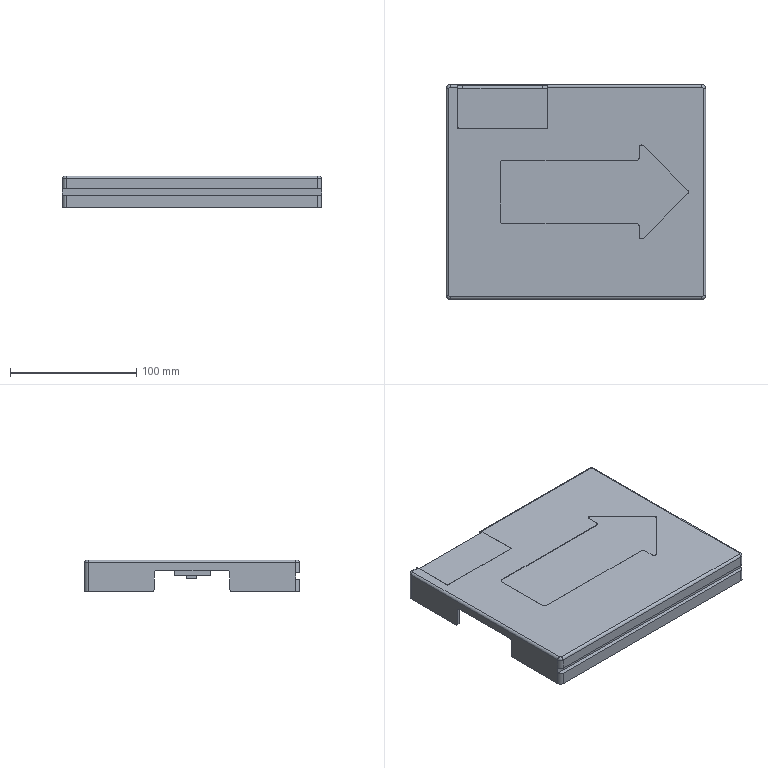NC program | NX | posted with a generic post | part box 205 x 170 x 25 mm
Lines 1 to 97 of 17262:
N10 G17 G21 G94 G90
(FLOOR_WALL_COPY , TOOL : D63)
N12 T03 M6
N14 G54
N16 G17 G0 G90 X-137. Y84.997 B0. C0. S6500 M3
N18 G43 Z30. H3
N20 Z7.03
N22 G94 G1 Z4.03 F1250.
N24 X-134.
N26 X134.
N28 Y36.731
N30 X-134.
N32 Y-11.534
N34 X134.
N36 Y-59.8
N38 X-134.
N40 X-137.
N42 Z7.03
N44 G0 Z30.
N46 Y84.997
N48 Z6.06
N50 G1 Z3.06
N52 X-134.
N54 X134.
N56 Y36.731
N58 X-134.
N60 Y-11.534
N62 X134.
N64 Y-59.8
N66 X-134.
N68 X-137.
N70 Z6.06
N72 G0 Z30.
N74 Y84.997
N76 Z5.09
N78 G1 Z2.09
N80 X-134.
N82 X134.
N84 Y36.731
N86 X-134.
N88 Y-11.534
N90 X134.
N92 Y-59.8
N94 X-134.
N96 X-137.
N98 Z5.09
N100 G0 Z30.
N102 Y84.997
N104 Z4.12
N106 G1 Z1.12
N108 X-134.
N110 X134.
N112 Y36.731
N114 X-134.
N116 Y-11.534
N118 X134.
N120 Y-59.8
N122 X-134.
N124 X-137.
N126 Z4.12
N128 G0 Z30.
N130 Y84.997
N132 Z3.15
N134 G1 Z0.15
N136 X-134.
N138 X134.
N140 Y36.731
N142 X-134.
N144 Y-11.534
N146 X134.
N148 Y-59.8
N150 X-134.
N152 X-137.
N154 Z3.15
N156 G0 Z30.
(FLOOR_WALL_COPY_1 , TOOL : D63)
N158 Y84.997
N160 Z3.
N162 G1 Z0.
N164 X-134.
N166 X134.
N168 Y36.731
N170 X-134.
N172 Y-11.534
N174 X134.
N176 Y-59.8
N178 X-134.
N180 X-137.
N182 Z3.
N184 G0 Z30.
N186 M5